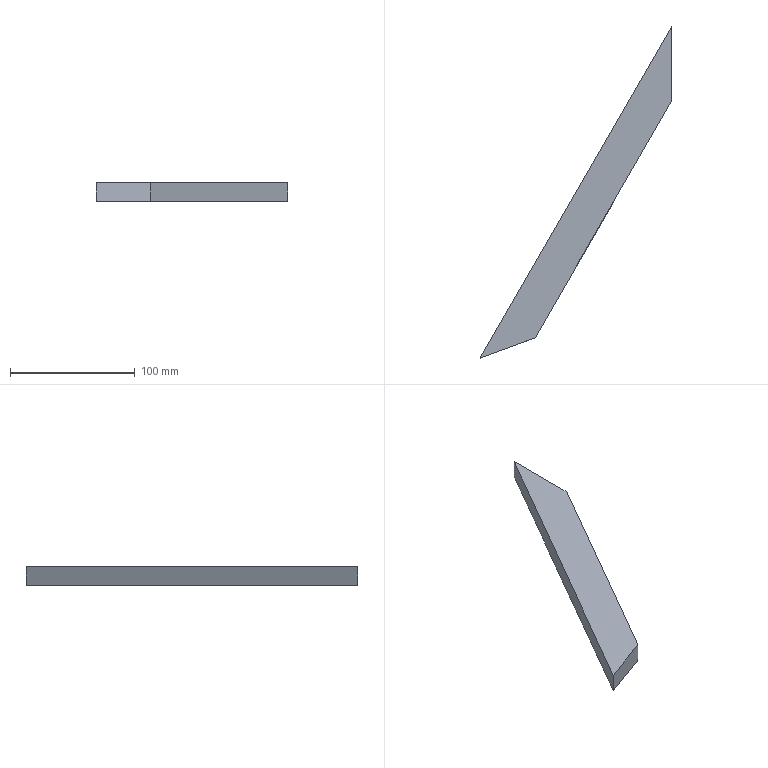Part | NX | features solid 2 | 1 solid | 6 faces | box 153.5 x 265.869 x 15 mm | volume 118414 mm3 | plane 6
STEP:
#1=CARTESIAN_POINT('',(540.357,-332.751,-30.));
#2=VERTEX_POINT('',#1);
#3=CARTESIAN_POINT('',(650.,-142.844,-30.));
#4=VERTEX_POINT('',#3);
#5=CARTESIAN_POINT('',(575.,-272.748,-30.));
#6=DIRECTION('',(-0.5,-0.866,0.));
#7=VECTOR('',#6,1000.);
#8=LINE('',#5,#7);
#9=EDGE_CURVE('',#2,#4,#8,.F.);
#10=ORIENTED_EDGE('',*,*,#9,.T.);
#11=CARTESIAN_POINT('',(650.,-142.844,-15.));
#12=VERTEX_POINT('',#11);
#13=CARTESIAN_POINT('',(650.,-142.844,0.));
#14=DIRECTION('',(0.,0.,-1.));
#15=VECTOR('',#14,1000.);
#16=LINE('',#13,#15);
#17=EDGE_CURVE('',#12,#4,#16,.T.);
#18=ORIENTED_EDGE('',*,*,#17,.F.);
#19=CARTESIAN_POINT('',(540.357,-332.751,-15.));
#20=VERTEX_POINT('',#19);
#21=CARTESIAN_POINT('',(575.,-272.748,-15.));
#22=DIRECTION('',(-0.5,-0.866,0.));
#23=VECTOR('',#22,1000.);
#24=LINE('',#21,#23);
#25=EDGE_CURVE('',#20,#12,#24,.F.);
#26=ORIENTED_EDGE('',*,*,#25,.F.);
#27=CARTESIAN_POINT('',(540.357,-332.751,0.));
#28=DIRECTION('',(0.,0.,-1.));
#29=VECTOR('',#28,1000.);
#30=LINE('',#27,#29);
#31=EDGE_CURVE('',#20,#2,#30,.T.);
#32=ORIENTED_EDGE('',*,*,#31,.T.);
#33=EDGE_LOOP('',(#10,#18,#26,#32));
#34=FACE_BOUND('',#33,.T.);
#35=CARTESIAN_POINT('',(575.,-272.748,0.));
#36=DIRECTION('',(0.866,-0.5,0.));
#37=DIRECTION('',(0.,0.,-1.));
#38=AXIS2_PLACEMENT_3D('',#35,#36,#37);
#39=PLANE('',#38);
#40=ADVANCED_FACE('',(#34),#39,.T.);
#41=ORIENTED_EDGE('',*,*,#25,.T.);
#42=CARTESIAN_POINT('',(650.,-82.844,-15.));
#43=VERTEX_POINT('',#42);
#44=CARTESIAN_POINT('',(650.,-30.,-15.));
#45=DIRECTION('',(0.,-1.,0.));
#46=VECTOR('',#45,1000.);
#47=LINE('',#44,#46);
#48=EDGE_CURVE('',#12,#43,#47,.F.);
#49=ORIENTED_EDGE('',*,*,#48,.T.);
#50=CARTESIAN_POINT('',(496.5,-348.714,-15.));
#51=VERTEX_POINT('',#50);
#52=CARTESIAN_POINT('',(549.019,-257.748,-15.));
#53=DIRECTION('',(0.5,0.866,0.));
#54=VECTOR('',#53,1000.);
#55=LINE('',#52,#54);
#56=EDGE_CURVE('',#51,#43,#55,.T.);
#57=ORIENTED_EDGE('',*,*,#56,.F.);
#58=CARTESIAN_POINT('',(690.261,-278.191,-15.));
#59=DIRECTION('',(0.9397,0.342,0.));
#60=VECTOR('',#59,1000.);
#61=LINE('',#58,#60);
#62=EDGE_CURVE('',#20,#51,#61,.F.);
#63=ORIENTED_EDGE('',*,*,#62,.F.);
#64=EDGE_LOOP('',(#41,#49,#57,#63));
#65=FACE_BOUND('',#64,.T.);
#66=CARTESIAN_POINT('',(575.,-272.748,-15.));
#67=DIRECTION('',(0.,0.,-1.));
#68=DIRECTION('',(-0.866,0.5,0.));
#69=AXIS2_PLACEMENT_3D('',#66,#67,#68);
#70=PLANE('',#69);
#71=ADVANCED_FACE('',(#65),#70,.F.);
#72=ORIENTED_EDGE('',*,*,#56,.T.);
#73=CARTESIAN_POINT('',(650.,-82.844,-30.));
#74=VERTEX_POINT('',#73);
#75=CARTESIAN_POINT('',(650.,-82.844,-25.));
#76=DIRECTION('',(0.,0.,1.));
#77=VECTOR('',#76,1000.);
#78=LINE('',#75,#77);
#79=EDGE_CURVE('',#43,#74,#78,.F.);
#80=ORIENTED_EDGE('',*,*,#79,.T.);
#81=CARTESIAN_POINT('',(496.5,-348.714,-30.));
#82=VERTEX_POINT('',#81);
#83=CARTESIAN_POINT('',(549.019,-257.748,-30.));
#84=DIRECTION('',(-0.5,-0.866,0.));
#85=VECTOR('',#84,1000.);
#86=LINE('',#83,#85);
#87=EDGE_CURVE('',#82,#74,#86,.F.);
#88=ORIENTED_EDGE('',*,*,#87,.F.);
#89=CARTESIAN_POINT('',(496.5,-348.714,-45.));
#90=DIRECTION('',(0.,0.,1.));
#91=VECTOR('',#90,1000.);
#92=LINE('',#89,#91);
#93=EDGE_CURVE('',#51,#82,#92,.F.);
#94=ORIENTED_EDGE('',*,*,#93,.F.);
#95=EDGE_LOOP('',(#72,#80,#88,#94));
#96=FACE_BOUND('',#95,.T.);
#97=CARTESIAN_POINT('',(549.019,-257.748,0.));
#98=DIRECTION('',(0.866,-0.5,0.));
#99=DIRECTION('',(0.,0.,-1.));
#100=AXIS2_PLACEMENT_3D('',#97,#98,#99);
#101=PLANE('',#100);
#102=ADVANCED_FACE('',(#96),#101,.F.);
#103=CARTESIAN_POINT('',(590.232,-314.598,-30.));
#104=DIRECTION('',(-0.9397,-0.342,0.));
#105=VECTOR('',#104,1000.);
#106=LINE('',#103,#105);
#107=EDGE_CURVE('',#2,#82,#106,.T.);
#108=ORIENTED_EDGE('',*,*,#107,.T.);
#109=ORIENTED_EDGE('',*,*,#87,.T.);
#110=CARTESIAN_POINT('',(650.,-272.748,-30.));
#111=DIRECTION('',(0.,1.,0.));
#112=VECTOR('',#111,1000.);
#113=LINE('',#110,#112);
#114=EDGE_CURVE('',#4,#74,#113,.T.);
#115=ORIENTED_EDGE('',*,*,#114,.F.);
#116=ORIENTED_EDGE('',*,*,#9,.F.);
#117=EDGE_LOOP('',(#108,#109,#115,#116));
#118=FACE_BOUND('',#117,.T.);
#119=CARTESIAN_POINT('',(575.,-272.748,-30.));
#120=DIRECTION('',(0.,0.,-1.));
#121=DIRECTION('',(-0.866,0.5,0.));
#122=AXIS2_PLACEMENT_3D('',#119,#120,#121);
#123=PLANE('',#122);
#124=ADVANCED_FACE('',(#118),#123,.T.);
#125=ORIENTED_EDGE('',*,*,#79,.F.);
#126=ORIENTED_EDGE('',*,*,#48,.F.);
#127=ORIENTED_EDGE('',*,*,#17,.T.);
#128=ORIENTED_EDGE('',*,*,#114,.T.);
#129=EDGE_LOOP('',(#125,#126,#127,#128));
#130=FACE_BOUND('',#129,.T.);
#131=CARTESIAN_POINT('',(650.,-30.,-25.));
#132=DIRECTION('',(-1.,0.,0.));
#133=DIRECTION('',(0.,-1.,0.));
#134=AXIS2_PLACEMENT_3D('',#131,#132,#133);
#135=PLANE('',#134);
#136=ADVANCED_FACE('',(#130),#135,.F.);
#137=ORIENTED_EDGE('',*,*,#93,.T.);
#138=ORIENTED_EDGE('',*,*,#107,.F.);
#139=ORIENTED_EDGE('',*,*,#31,.F.);
#140=ORIENTED_EDGE('',*,*,#62,.T.);
#141=EDGE_LOOP('',(#137,#138,#139,#140));
#142=FACE_BOUND('',#141,.T.);
#143=CARTESIAN_POINT('',(690.261,-278.191,-45.));
#144=DIRECTION('',(0.342,-0.9397,0.));
#145=DIRECTION('',(-0.9397,-0.342,0.));
#146=AXIS2_PLACEMENT_3D('',#143,#144,#145);
#147=PLANE('',#146);
#148=ADVANCED_FACE('',(#142),#147,.T.);
#149=CLOSED_SHELL('',(#40,#71,#102,#124,#136,#148));
#150=MANIFOLD_SOLID_BREP('',#149);
#151=(LENGTH_UNIT()NAMED_UNIT(*)SI_UNIT(.MILLI.,.METRE.));
#152=UNCERTAINTY_MEASURE_WITH_UNIT(LENGTH_MEASURE(0.00001),#151,'','');
#153=(NAMED_UNIT(*)PLANE_ANGLE_UNIT()SI_UNIT($,.RADIAN.));
#154=(NAMED_UNIT(*)SI_UNIT($,.STERADIAN.)SOLID_ANGLE_UNIT());
#155=(GEOMETRIC_REPRESENTATION_CONTEXT(3)GLOBAL_UNCERTAINTY_ASSIGNED_CONTEXT((#152))GLOBAL_UNIT_ASSIGNED_CONTEXT((#151,#153,#154))REPRESENTATION_CONTEXT('',''));
#156=ADVANCED_BREP_SHAPE_REPRESENTATION('',(#150),#155);